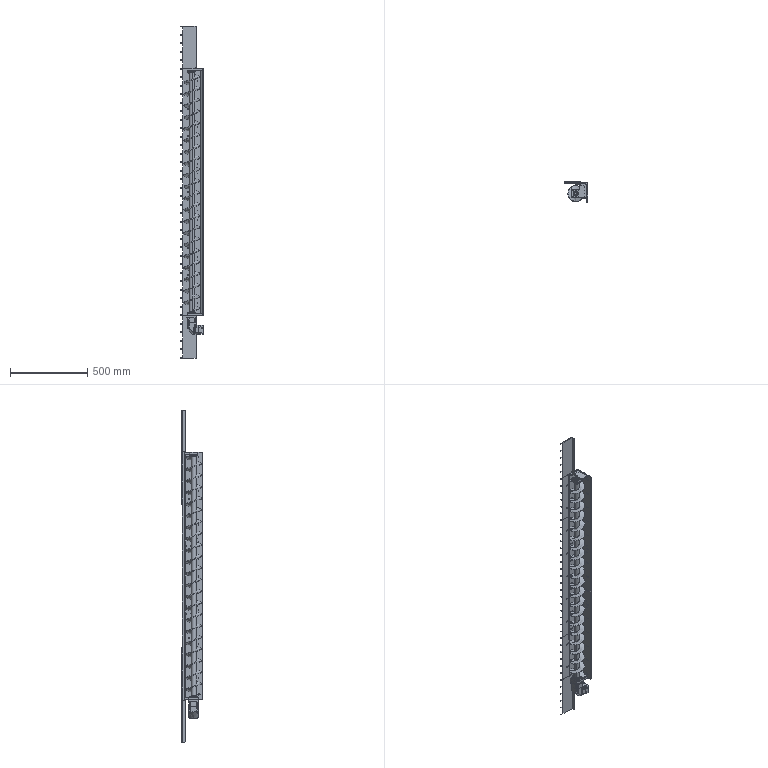Part | SolidWorks | 25 solids | 1366 faces | box 150 x 131 x 2150 mm | volume 4854197 mm3 | cylinder 612 | plane 566 | cone 111 | spline 53 | torus 24 | commonest cylinder face diameters 4.2 x190 5.8 x42 5.5 x40 10 x32 10.1 x30 69 x26